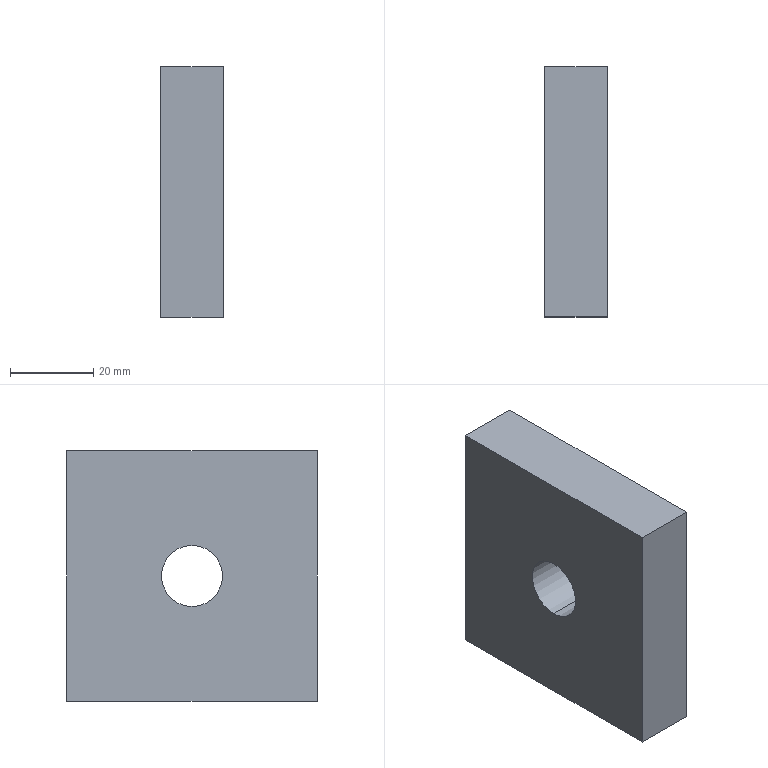Part | NX | 1 solid | 8 faces | box 15 x 60 x 60 mm | volume 51475 mm3 | plane 6 | cylinder 2 | commonest cylinder face diameters 14.64 x2
STEP:
#1=CARTESIAN_POINT('',(-250.326,-649.499,2417.766));
#2=VERTEX_POINT('',#1);
#3=CARTESIAN_POINT('',(-250.326,-649.499,2432.406));
#4=VERTEX_POINT('',#3);
#5=CARTESIAN_POINT('',(-250.326,-649.499,2425.086));
#6=DIRECTION('',(-1.,0.,0.));
#7=DIRECTION('',(0.,0.,1.));
#8=AXIS2_PLACEMENT_3D('',#5,#6,#7);
#9=CIRCLE('',#8,7.32);
#10=EDGE_CURVE('',#2,#4,#9,.T.);
#11=ORIENTED_EDGE('',*,*,#10,.T.);
#12=CARTESIAN_POINT('',(-235.326,-649.499,2432.406));
#13=VERTEX_POINT('',#12);
#14=CARTESIAN_POINT('',(-250.326,-649.499,2432.406));
#15=DIRECTION('',(1.,0.,0.));
#16=VECTOR('',#15,1.);
#17=LINE('',#14,#16);
#18=EDGE_CURVE('',#4,#13,#17,.T.);
#19=ORIENTED_EDGE('',*,*,#18,.T.);
#20=CARTESIAN_POINT('',(-235.326,-649.499,2417.766));
#21=VERTEX_POINT('',#20);
#22=CARTESIAN_POINT('',(-235.326,-649.499,2425.086));
#23=DIRECTION('',(-1.,0.,0.));
#24=DIRECTION('',(0.,0.,1.));
#25=AXIS2_PLACEMENT_3D('',#22,#23,#24);
#26=CIRCLE('',#25,7.32);
#27=EDGE_CURVE('',#21,#13,#26,.T.);
#28=ORIENTED_EDGE('',*,*,#27,.F.);
#29=CARTESIAN_POINT('',(-250.326,-649.499,2417.766));
#30=DIRECTION('',(-1.,0.,0.));
#31=VECTOR('',#30,1.);
#32=LINE('',#29,#31);
#33=EDGE_CURVE('',#21,#2,#32,.T.);
#34=ORIENTED_EDGE('',*,*,#33,.T.);
#35=EDGE_LOOP('',(#11,#19,#28,#34));
#36=FACE_OUTER_BOUND('',#35,.T.);
#37=CARTESIAN_POINT('',(-250.326,-649.499,2425.086));
#38=DIRECTION('',(1.,0.,0.));
#39=DIRECTION('',(0.,0.,-1.));
#40=AXIS2_PLACEMENT_3D('',#37,#38,#39);
#41=CYLINDRICAL_SURFACE('',#40,7.32);
#42=ADVANCED_FACE('',(#36),#41,.F.);
#43=CARTESIAN_POINT('',(-250.326,-619.499,2395.086));
#44=VERTEX_POINT('',#43);
#45=CARTESIAN_POINT('',(-250.326,-679.499,2395.086));
#46=VERTEX_POINT('',#45);
#47=CARTESIAN_POINT('',(-250.326,-619.499,2395.086));
#48=DIRECTION('',(0.,-1.,0.));
#49=VECTOR('',#48,1.);
#50=LINE('',#47,#49);
#51=EDGE_CURVE('',#44,#46,#50,.T.);
#52=ORIENTED_EDGE('',*,*,#51,.T.);
#53=CARTESIAN_POINT('',(-250.326,-679.499,2455.086));
#54=VERTEX_POINT('',#53);
#55=CARTESIAN_POINT('',(-250.326,-679.499,2395.086));
#56=DIRECTION('',(0.,0.,1.));
#57=VECTOR('',#56,1.);
#58=LINE('',#55,#57);
#59=EDGE_CURVE('',#46,#54,#58,.T.);
#60=ORIENTED_EDGE('',*,*,#59,.T.);
#61=CARTESIAN_POINT('',(-250.326,-619.499,2455.086));
#62=VERTEX_POINT('',#61);
#63=CARTESIAN_POINT('',(-250.326,-619.499,2455.086));
#64=DIRECTION('',(0.,1.,0.));
#65=VECTOR('',#64,1.);
#66=LINE('',#63,#65);
#67=EDGE_CURVE('',#54,#62,#66,.T.);
#68=ORIENTED_EDGE('',*,*,#67,.T.);
#69=CARTESIAN_POINT('',(-250.326,-619.499,2395.086));
#70=DIRECTION('',(0.,0.,-1.));
#71=VECTOR('',#70,1.);
#72=LINE('',#69,#71);
#73=EDGE_CURVE('',#62,#44,#72,.T.);
#74=ORIENTED_EDGE('',*,*,#73,.T.);
#75=EDGE_LOOP('',(#52,#60,#68,#74));
#76=FACE_BOUND('',#75,.T.);
#77=ORIENTED_EDGE('',*,*,#10,.F.);
#78=CARTESIAN_POINT('',(-250.326,-649.499,2425.086));
#79=DIRECTION('',(-1.,0.,0.));
#80=DIRECTION('',(0.,0.,1.));
#81=AXIS2_PLACEMENT_3D('',#78,#79,#80);
#82=CIRCLE('',#81,7.32);
#83=EDGE_CURVE('',#4,#2,#82,.T.);
#84=ORIENTED_EDGE('',*,*,#83,.F.);
#85=EDGE_LOOP('',(#77,#84));
#86=FACE_BOUND('',#85,.T.);
#87=CARTESIAN_POINT('',(-250.326,-679.499,2395.086));
#88=DIRECTION('',(-1.,0.,0.));
#89=DIRECTION('',(0.,0.,1.));
#90=AXIS2_PLACEMENT_3D('',#87,#88,#89);
#91=PLANE('',#90);
#92=ADVANCED_FACE('',(#76,#86),#91,.T.);
#93=CARTESIAN_POINT('',(-235.326,-619.499,2395.086));
#94=VERTEX_POINT('',#93);
#95=CARTESIAN_POINT('',(-235.326,-679.499,2395.086));
#96=VERTEX_POINT('',#95);
#97=CARTESIAN_POINT('',(-235.326,-619.499,2395.086));
#98=DIRECTION('',(0.,-1.,0.));
#99=VECTOR('',#98,1.);
#100=LINE('',#97,#99);
#101=EDGE_CURVE('',#94,#96,#100,.T.);
#102=ORIENTED_EDGE('',*,*,#101,.F.);
#103=CARTESIAN_POINT('',(-235.326,-619.499,2455.086));
#104=VERTEX_POINT('',#103);
#105=CARTESIAN_POINT('',(-235.326,-619.499,2395.086));
#106=DIRECTION('',(0.,0.,-1.));
#107=VECTOR('',#106,1.);
#108=LINE('',#105,#107);
#109=EDGE_CURVE('',#104,#94,#108,.T.);
#110=ORIENTED_EDGE('',*,*,#109,.F.);
#111=CARTESIAN_POINT('',(-235.326,-679.499,2455.086));
#112=VERTEX_POINT('',#111);
#113=CARTESIAN_POINT('',(-235.326,-619.499,2455.086));
#114=DIRECTION('',(0.,1.,0.));
#115=VECTOR('',#114,1.);
#116=LINE('',#113,#115);
#117=EDGE_CURVE('',#112,#104,#116,.T.);
#118=ORIENTED_EDGE('',*,*,#117,.F.);
#119=CARTESIAN_POINT('',(-235.326,-679.499,2395.086));
#120=DIRECTION('',(0.,0.,1.));
#121=VECTOR('',#120,1.);
#122=LINE('',#119,#121);
#123=EDGE_CURVE('',#96,#112,#122,.T.);
#124=ORIENTED_EDGE('',*,*,#123,.F.);
#125=EDGE_LOOP('',(#102,#110,#118,#124));
#126=FACE_BOUND('',#125,.T.);
#127=ORIENTED_EDGE('',*,*,#27,.T.);
#128=CARTESIAN_POINT('',(-235.326,-649.499,2425.086));
#129=DIRECTION('',(-1.,0.,0.));
#130=DIRECTION('',(0.,0.,1.));
#131=AXIS2_PLACEMENT_3D('',#128,#129,#130);
#132=CIRCLE('',#131,7.32);
#133=EDGE_CURVE('',#13,#21,#132,.T.);
#134=ORIENTED_EDGE('',*,*,#133,.T.);
#135=EDGE_LOOP('',(#127,#134));
#136=FACE_BOUND('',#135,.T.);
#137=CARTESIAN_POINT('',(-235.326,-679.499,2395.086));
#138=DIRECTION('',(-1.,0.,0.));
#139=DIRECTION('',(0.,0.,1.));
#140=AXIS2_PLACEMENT_3D('',#137,#138,#139);
#141=PLANE('',#140);
#142=ADVANCED_FACE('',(#126,#136),#141,.F.);
#143=ORIENTED_EDGE('',*,*,#101,.T.);
#144=CARTESIAN_POINT('',(-250.326,-679.499,2395.086));
#145=DIRECTION('',(1.,0.,0.));
#146=VECTOR('',#145,1.);
#147=LINE('',#144,#146);
#148=EDGE_CURVE('',#46,#96,#147,.T.);
#149=ORIENTED_EDGE('',*,*,#148,.F.);
#150=ORIENTED_EDGE('',*,*,#51,.F.);
#151=CARTESIAN_POINT('',(-250.326,-619.499,2395.086));
#152=DIRECTION('',(1.,0.,0.));
#153=VECTOR('',#152,1.);
#154=LINE('',#151,#153);
#155=EDGE_CURVE('',#44,#94,#154,.T.);
#156=ORIENTED_EDGE('',*,*,#155,.T.);
#157=EDGE_LOOP('',(#143,#149,#150,#156));
#158=FACE_OUTER_BOUND('',#157,.T.);
#159=CARTESIAN_POINT('',(-250.326,-619.499,2395.086));
#160=DIRECTION('',(0.,0.,1.));
#161=DIRECTION('',(0.,-1.,0.));
#162=AXIS2_PLACEMENT_3D('',#159,#160,#161);
#163=PLANE('',#162);
#164=ADVANCED_FACE('',(#158),#163,.F.);
#165=ORIENTED_EDGE('',*,*,#123,.T.);
#166=CARTESIAN_POINT('',(-250.326,-679.499,2455.086));
#167=DIRECTION('',(1.,0.,0.));
#168=VECTOR('',#167,1.);
#169=LINE('',#166,#168);
#170=EDGE_CURVE('',#54,#112,#169,.T.);
#171=ORIENTED_EDGE('',*,*,#170,.F.);
#172=ORIENTED_EDGE('',*,*,#59,.F.);
#173=ORIENTED_EDGE('',*,*,#148,.T.);
#174=EDGE_LOOP('',(#165,#171,#172,#173));
#175=FACE_OUTER_BOUND('',#174,.T.);
#176=CARTESIAN_POINT('',(-250.326,-679.499,2395.086));
#177=DIRECTION('',(0.,1.,0.));
#178=DIRECTION('',(0.,0.,1.));
#179=AXIS2_PLACEMENT_3D('',#176,#177,#178);
#180=PLANE('',#179);
#181=ADVANCED_FACE('',(#175),#180,.F.);
#182=ORIENTED_EDGE('',*,*,#117,.T.);
#183=CARTESIAN_POINT('',(-250.326,-619.499,2455.086));
#184=DIRECTION('',(1.,0.,0.));
#185=VECTOR('',#184,1.);
#186=LINE('',#183,#185);
#187=EDGE_CURVE('',#62,#104,#186,.T.);
#188=ORIENTED_EDGE('',*,*,#187,.F.);
#189=ORIENTED_EDGE('',*,*,#67,.F.);
#190=ORIENTED_EDGE('',*,*,#170,.T.);
#191=EDGE_LOOP('',(#182,#188,#189,#190));
#192=FACE_OUTER_BOUND('',#191,.T.);
#193=CARTESIAN_POINT('',(-250.326,-619.499,2455.086));
#194=DIRECTION('',(0.,0.,-1.));
#195=DIRECTION('',(-1.,0.,0.));
#196=AXIS2_PLACEMENT_3D('',#193,#194,#195);
#197=PLANE('',#196);
#198=ADVANCED_FACE('',(#192),#197,.F.);
#199=ORIENTED_EDGE('',*,*,#109,.T.);
#200=ORIENTED_EDGE('',*,*,#155,.F.);
#201=ORIENTED_EDGE('',*,*,#73,.F.);
#202=ORIENTED_EDGE('',*,*,#187,.T.);
#203=EDGE_LOOP('',(#199,#200,#201,#202));
#204=FACE_OUTER_BOUND('',#203,.T.);
#205=CARTESIAN_POINT('',(-250.326,-619.499,2395.086));
#206=DIRECTION('',(0.,-1.,0.));
#207=DIRECTION('',(0.,0.,-1.));
#208=AXIS2_PLACEMENT_3D('',#205,#206,#207);
#209=PLANE('',#208);
#210=ADVANCED_FACE('',(#204),#209,.F.);
#211=ORIENTED_EDGE('',*,*,#18,.F.);
#212=ORIENTED_EDGE('',*,*,#83,.T.);
#213=ORIENTED_EDGE('',*,*,#33,.F.);
#214=ORIENTED_EDGE('',*,*,#133,.F.);
#215=EDGE_LOOP('',(#211,#212,#213,#214));
#216=FACE_OUTER_BOUND('',#215,.T.);
#217=CARTESIAN_POINT('',(-250.326,-649.499,2425.086));
#218=DIRECTION('',(1.,0.,0.));
#219=DIRECTION('',(0.,0.,-1.));
#220=AXIS2_PLACEMENT_3D('',#217,#218,#219);
#221=CYLINDRICAL_SURFACE('',#220,7.32);
#222=ADVANCED_FACE('',(#216),#221,.F.);
#223=CLOSED_SHELL('',(#42,#92,#142,#164,#181,#198,#210,#222));
#224=MANIFOLD_SOLID_BREP('',#223);
#225=(LENGTH_UNIT()NAMED_UNIT(*)SI_UNIT(.MILLI.,.METRE.));
#226=UNCERTAINTY_MEASURE_WITH_UNIT(LENGTH_MEASURE(0.00002),#225,'','');
#227=(NAMED_UNIT(*)PLANE_ANGLE_UNIT()SI_UNIT($,.RADIAN.));
#228=PLANE_ANGLE_MEASURE_WITH_UNIT(PLANE_ANGLE_MEASURE(0.01745),#227);
#229=DIMENSIONAL_EXPONENTS(0.,0.,0.,0.,0.,0.,0.);
#230=(CONVERSION_BASED_UNIT('DEGREE',#228)NAMED_UNIT(#229)PLANE_ANGLE_UNIT());
#231=(NAMED_UNIT(*)SI_UNIT($,.STERADIAN.)SOLID_ANGLE_UNIT());
#232=(GEOMETRIC_REPRESENTATION_CONTEXT(3)GLOBAL_UNCERTAINTY_ASSIGNED_CONTEXT((#226))GLOBAL_UNIT_ASSIGNED_CONTEXT((#225,#230,#231))REPRESENTATION_CONTEXT('',''));
#233=ADVANCED_BREP_SHAPE_REPRESENTATION('',(#224),#232);